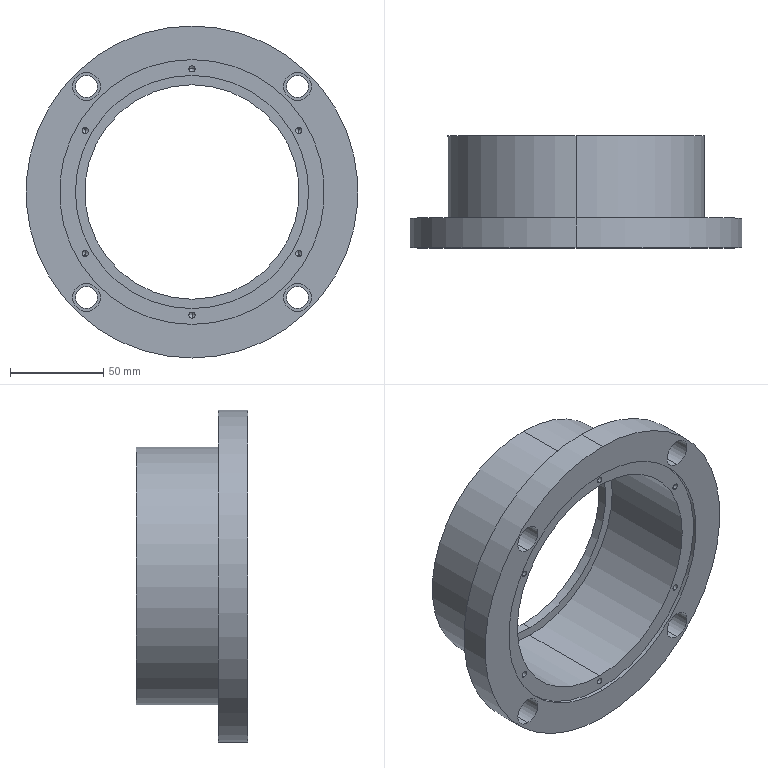Part | SolidWorks | features BaseBody 1 | 1 solid | 59 faces | box 178 x 60 x 178 mm | volume 311606 mm3 | cylinder 38 | cone 12 | plane 9 | commonest cylinder face diameters 3.3 x12 12 x8 15 x8 115 x2 125 x2 138 x2